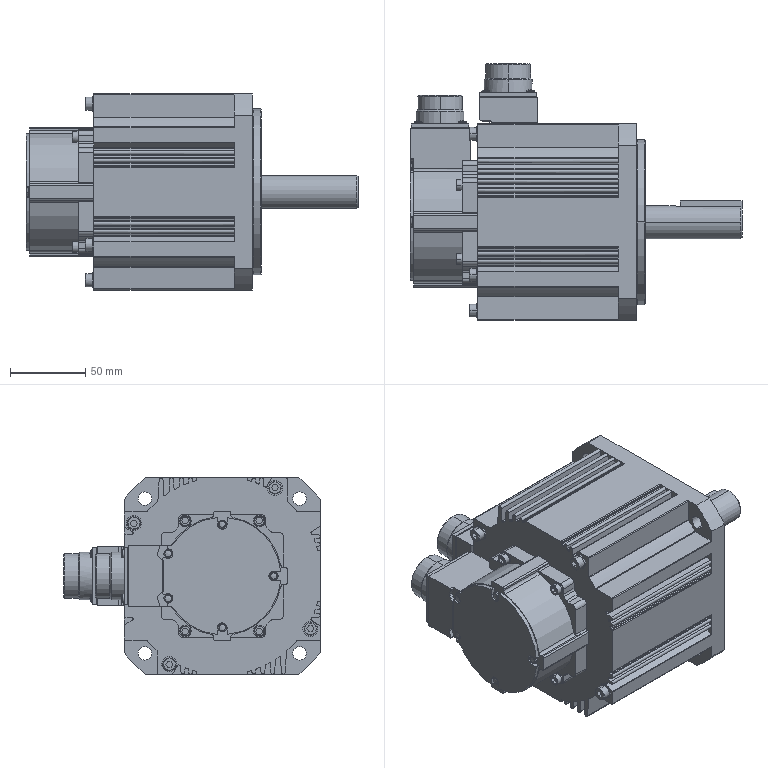Part | SolidWorks | 1 solid | 668 faces | box 220 x 170 x 130 mm | volume 1941272 mm3 | cylinder 305 | plane 268 | cone 49 | torus 33 | sphere 13 | commonest cylinder face diameters 1 x90 2 x30 131 x24 2.5 x22 4 x20 5.6 x10